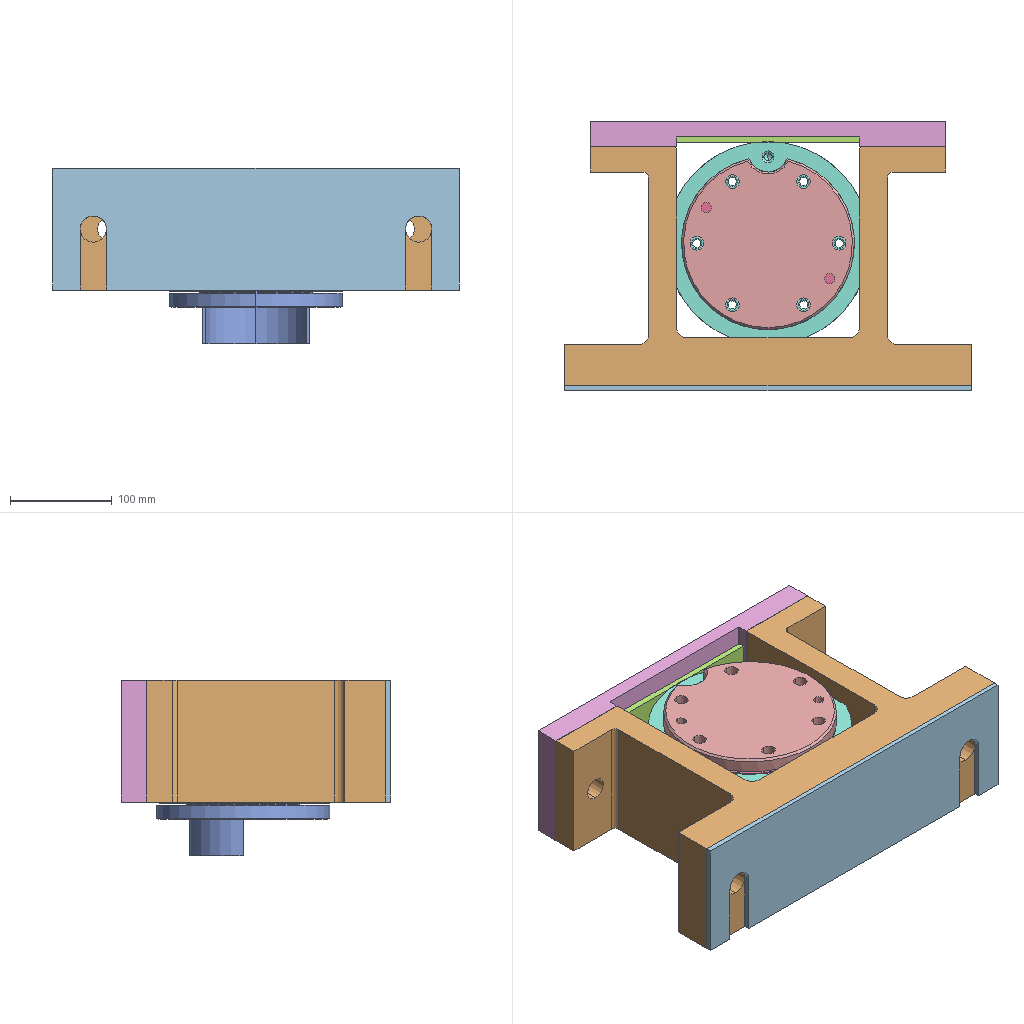Assembly | SolidWorks | 10 different items | 12 placed | box 400 x 265 x 173 mm
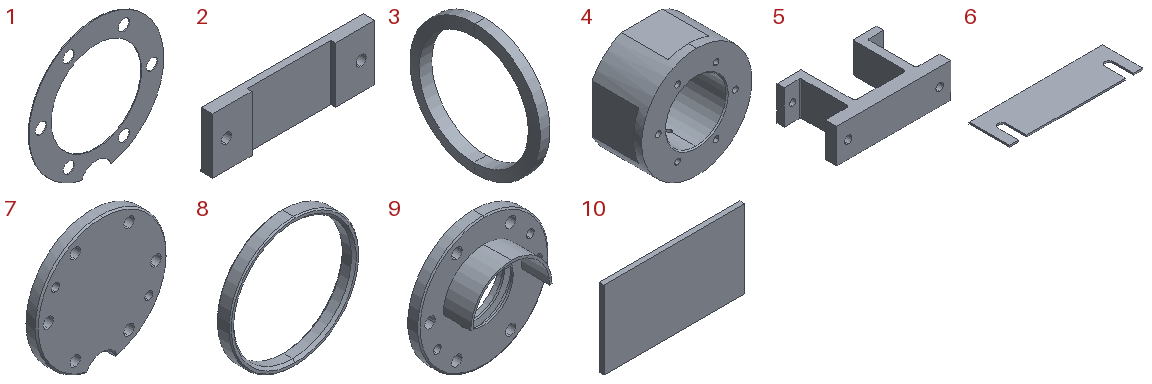Parts list (item | quantity | size | volume | features):
1 | x2 | 170 x 1 x 167.917 mm | 11164 mm3 | features Extrusion 1
2 | x1 | 350 x 25 x 120 mm | 815006 mm3 | features ICE 2, Extrusion 1, Fillet 1
3 | x1 | 8.842 x 92 x 92 mm | 15716 mm3 | features Sweep 1
4 | x1 | 200 x 100 x 200 mm | 2011529 mm3 | features HoleWzd 5, ICE 3, 3DProfileFeature 1, Chamfer 1, CirPattern 1, Extrusion 1, Fillet 1
5 | x1 | 400 x 235 x 120 mm | 3581826 mm3 | features ICE 3, Extrusion 1
6 | x1 | 400 x 120 x 5 mm | 221745 mm3 | features Extrusion 1, ICE 1
7 | x1 | 170 x 28 x 167.917 mm | 262504 mm3 | features ICE 3, Chamfer 2, Fillet 2, Extrusion 1, HoleWzd 1
8 | x2 | 110 x 11.75 x 110 mm | 17763 mm3 | features Chamfer 2, Extrusion 1
9 | x1 | 170 x 64 x 170 mm | 268447 mm3 | features ICE 3, Chamfer 2, Fillet 2, CirPattern 1, Extrusion 1, HoleWzd 1, RevCut 1
10 | x1 | 180 x 6 x 100 mm | 108000 mm3 | features Extrusion 1
Mates (type | each side: item.copy, entity, surface, feature):
Concentric | 4.1 face cylinder Boss-Extrude1 | 5.1 edge
Concentric | 7.1 face cylinder Cut-Extrude2 | 4.1 face cylinder CirPattern1
Concentric | 9.1 face cylinder CirPattern1 | 4.1 face cylinder M12 Tapped Hole2
Concentric | 2.1 face cylinder Cut-Extrude2 | 5.1 face cylinder Cut-Extrude2 | 2 times
Coincident | 10.1 face plane Boss-Extrude1 | 2.1 face plane Cut-Extrude1 | 2 times
Coincident | 10.1 face plane Boss-Extrude1 | 2.1 face plane Boss-Extrude1
Coincident | 4.1 face plane Cut-Extrude1 | 5.1 face plane Boss-Extrude1
Coincident | 4.1 face plane Cut-Extrude1 | 5.1 face plane Cut-Extrude3
Coincident | 2.1 face plane Boss-Extrude1 | 5.1 face plane Boss-Extrude1
DistanceDim | 9.1 face plane Boss-Extrude1 | 4.1 face plane Boss-Extrude1
DistanceDim | 4.1 face plane Boss-Extrude1 | 7.1 face plane Boss-Extrude1
Concentric | 8.1 face cylinder Boss-Extrude1 | 8.2 face cylinder Boss-Extrude1
Coincident | 8.1 face plane Boss-Extrude1 | 8.2 face plane Boss-Extrude1
Coincident | 7.1 face plane Boss-Extrude2 | 8.2 face plane Boss-Extrude1
Concentric | 9.1 face cylinder Boss-Extrude1 | 3.1 face cylinder Sweep1
Coincident | 9.1 face cone Cut-Revolve1 | 3.1 face cone Sweep1
Coincident | 4.1 face plane Boss-Extrude1 | 1.1 face plane Boss-Extrude1
Concentric | 7.1 face cylinder Cut-Extrude2 | 1.1 face cylinder Boss-Extrude1
Coincident | 4.1 face plane Boss-Extrude1 | 1.2 face plane Boss-Extrude1
Coincident | 5.1 face plane Boss-Extrude1 | 6.1 face plane Boss-Extrude1 | 3 times